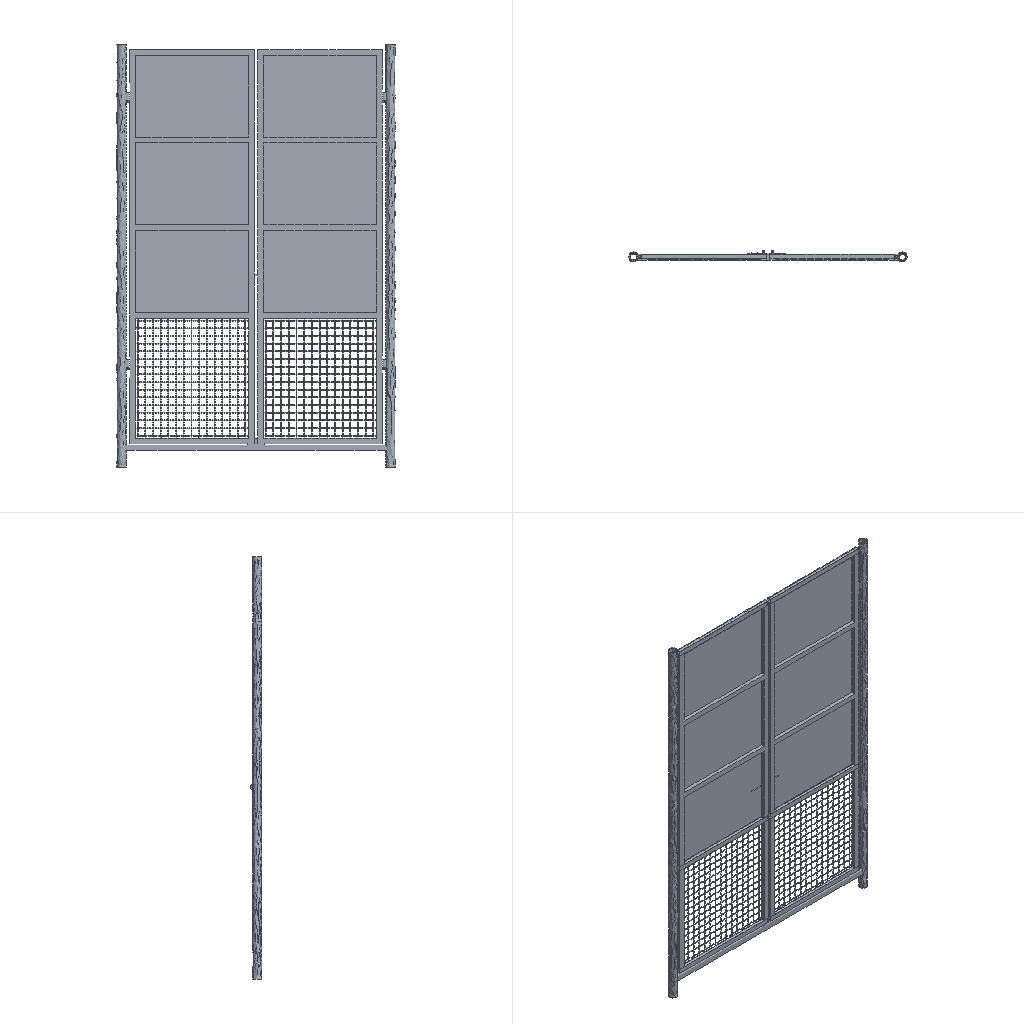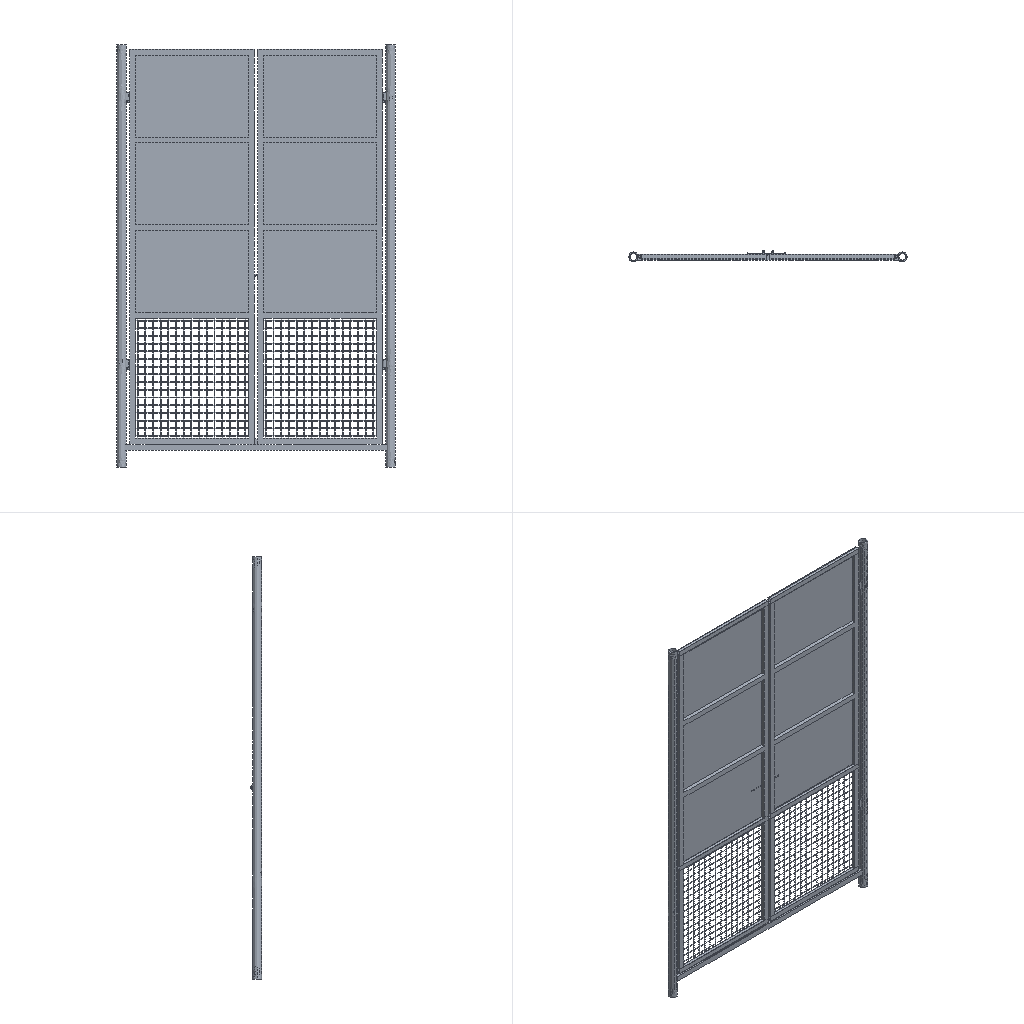Simulation study | ansys workbench
Set-up summary:
category,name,step,type,value,unit,region
solver,ansys_workbench
units,mm-N-s-tonne (MPa),,stated,"/units,MPA"
analysis,deck-1/LS1,,static
load_step,deck-1/LS1,deck-1/LS1,static,nsubst=1; time=1
analysis,deck-2/LS1,,static
load_step,deck-2/LS1,deck-2/LS1,static,nsubst=5; time=1
mesh,deck-1.dat,,nodes,113582
mesh,deck-1.dat,,elements,62853
element_type,SOLID187,,,49263,,deck-1.dat
element_type,SURF154,,,10352,,deck-1.dat
element_type,TARGE170,,,1619,,deck-1.dat
element_type,CONTA174,,,1619,,deck-1.dat
mesh,deck-2.dat,,nodes,260100
mesh,deck-2.dat,,elements,139136
element_type,SOLID187,,,123421,,deck-2.dat
element_type,CONTA174,,,8023,,deck-2.dat
element_type,TARGE170,,,7648,,deck-2.dat
element_type,SURF154,,,44,,deck-2.dat
material,Structural Steel,,E,200000,tonne s^-2 mm^-1
material,Structural Steel,,nu,0.3
material,Structural Steel,,density,7.85e-09,tonne mm^-3
material,Structural Steel,,conductivity,60.5,tonne mm s^-3 C^-1
material,Structural Steel,,specific_heat,4.34e+08,mm^2 s^-2 C^-1
material,Structural Steel,,cte,1.2e-05,C^-1
material,Structural Steel,,permeability,10000
material,Structural Steel,,resistivity,0.00017,ohm mm
load,Define Force Using Surface Effect Elements,deck-1/LS1,surface-effect pres face 2,-0.000148,,SURF154 #23
load,Define Force Using Surface Effect Elements,deck-2/LS1,surface-effect pres face 2,0.06,,SURF154 #18
bc,Fixed Supports,deck-1/model,fixed,[dofs=ALL],,_FIXEDSU
bc,Fixed Supports,deck-2/model,fixed,[dofs=ALL],,_FIXEDSU
contact,Contact Region 7,,bonded (always),element=CONTA174
contact,Contact Region 8,,bonded (always),element=CONTA174
contact,Contact Region 9,,bonded (always),element=CONTA174
contact,Contact Region 14,,bonded (always),element=CONTA174
contact,Contact Region 21,,bonded (always),element=CONTA174
contact,Contact Region 22,,bonded (always),element=CONTA174
contact,Contact Region 27,,bonded (always),element=CONTA174
contact,Contact Region 28,,bonded (always),element=CONTA174
contact,Frictional - SYS-FreeParts|NONE[16] ? SYS-FreeParts|NONE[18],,standard (frictionless/frictional),friction=0.2; element=CONTA174
contact,Frictional - SYS-FreeParts|NONE[17] ? SYS-FreeParts|NONE[13],,standard (frictionless/frictional),element=CONTA174
contact,Frictional - SYS-FreeParts|NONE[14] ? ?,,standard (frictionless/frictional),friction=0.6; element=CONTA174
contact,Frictional - SYS-FreeParts|NONE[15] ? ?,,standard (frictionless/frictional),element=CONTA174
contact,contact 5,,bonded (always),element=CONTA174
named_set,_FIXEDSU,,node,414
named_set,_FIXEDSU,,node,264
Results summary:
result,analyses[0].index,,,1
result,analyses[0].system,,,SYS
result,analyses[0].deck,,,deck-1.dat
result,analyses[0].solve_status,,,completed
result,analyses[0].analysis_type,,,static
result,analyses[0].physics,,,mechanical
result,analyses[0].unit_system,,,"NMM: mm, ton, N, s, mV, mA, degC"
result,analyses[0].n_sets,,,1
result,analyses[0].load_steps[0].set,set=1,,1
result,analyses[0].load_steps[0].time_or_freq,set=1,,1
result,analyses[0].load_steps[0].max_displacement_magnitude,set=1,,2.473
result,analyses[0].load_steps[0].max_von_mises_nodal,set=1,,75.69
result,analyses[0].load_steps[0].reaction_force_sum_xyz[1],set=1,,-2.97186e-06
result,analyses[0].load_steps[0].reaction_force_sum_xyz[2],set=1,,300
result,analyses[0].load_steps[0].reaction_force_sum_xyz[3],set=1,,8.42152e-06
result,analyses[1].index,,,2
result,analyses[1].system,,,SYS-1
result,analyses[1].deck,,,deck-2.dat
result,analyses[1].solve_status,,,completed
result,analyses[1].analysis_type,,,static
result,analyses[1].physics,,,mechanical
result,analyses[1].unit_system,,,"NMM: mm, ton, N, s, mV, mA, degC"
result,analyses[1].n_sets,,,4
result,analyses[1].load_steps[0].set,set=4,,4
result,analyses[1].load_steps[0].time_or_freq,set=4,,1
result,analyses[1].load_steps[0].max_displacement_magnitude,set=4,,344.602
result,analyses[1].load_steps[0].max_von_mises_nodal,set=4,,7419.38
result,analyses[1].load_steps[0].reaction_force_sum_xyz[1],set=4,,301.494
result,analyses[1].load_steps[0].reaction_force_sum_xyz[2],set=4,,-133.111
result,analyses[1].load_steps[0].reaction_force_sum_xyz[3],set=4,,0.05161
result,geometry_export[0][0],,,.step
result,geometry_export[0][1],,,ok
result,geometry_export[0][2],,,18